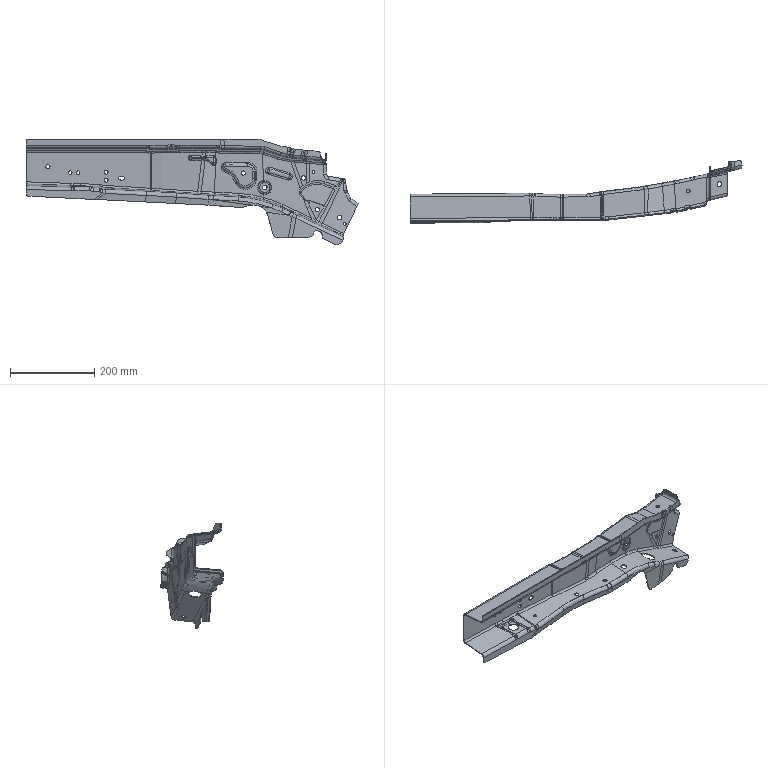Part | 1 solid | 815 faces | box 789.751 x 148.694 x 250.646 mm | volume 403377 mm3 | spline 527 | cylinder 202 | plane 65 | other 10 | sphere 6 | torus 5 | commonest cylinder face diameters 16 x32 10 x26 12 x25 14 x17 20 x13 9 x12